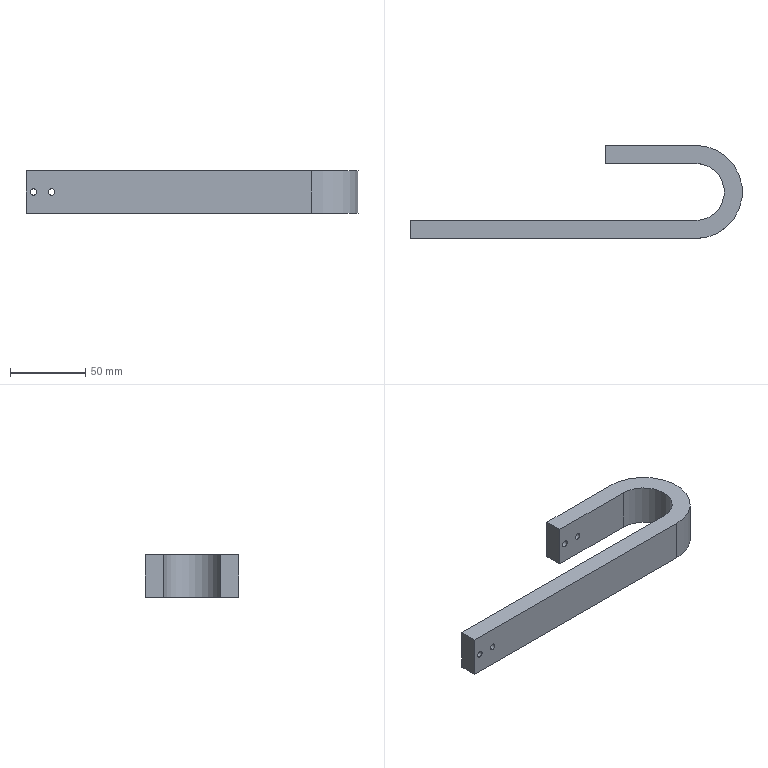Part | NX | features BREP 1 | 1 solid | 18 faces | box 221 x 62 x 28 mm | volume 109724 mm3 | cylinder 10 | plane 8 | commonest cylinder face diameters 4.2 x8 38 x1 62 x1
STEP:
#1=CARTESIAN_POINT('',(280.442,-89.817,14.));
#2=VERTEX_POINT('',#1);
#3=CARTESIAN_POINT('',(276.242,-89.817,14.));
#4=VERTEX_POINT('',#3);
#5=CARTESIAN_POINT('',(278.342,-89.817,14.));
#6=DIRECTION('',(0.,1.,0.));
#7=DIRECTION('',(-1.,0.,0.));
#8=AXIS2_PLACEMENT_3D('',#5,#6,#7);
#9=CIRCLE('',#8,2.1);
#10=EDGE_CURVE('',#2,#4,#9,.T.);
#11=ORIENTED_EDGE('',*,*,#10,.F.);
#12=CARTESIAN_POINT('',(280.442,-77.817,14.));
#13=VERTEX_POINT('',#12);
#14=CARTESIAN_POINT('',(280.442,-92.817,14.));
#15=DIRECTION('',(0.,1.,0.));
#16=VECTOR('',#15,1000.);
#17=LINE('',#14,#16);
#18=EDGE_CURVE('',#2,#13,#17,.T.);
#19=ORIENTED_EDGE('',*,*,#18,.T.);
#20=CARTESIAN_POINT('',(276.242,-77.817,14.));
#21=VERTEX_POINT('',#20);
#22=CARTESIAN_POINT('',(278.342,-77.817,14.));
#23=DIRECTION('',(0.,1.,0.));
#24=DIRECTION('',(-1.,0.,0.));
#25=AXIS2_PLACEMENT_3D('',#22,#23,#24);
#26=CIRCLE('',#25,2.1);
#27=EDGE_CURVE('',#13,#21,#26,.T.);
#28=ORIENTED_EDGE('',*,*,#27,.T.);
#29=CARTESIAN_POINT('',(276.242,-92.817,14.));
#30=DIRECTION('',(0.,1.,0.));
#31=VECTOR('',#30,1000.);
#32=LINE('',#29,#31);
#33=EDGE_CURVE('',#4,#21,#32,.T.);
#34=ORIENTED_EDGE('',*,*,#33,.F.);
#35=EDGE_LOOP('',(#11,#19,#28,#34));
#36=FACE_BOUND('',#35,.T.);
#37=CARTESIAN_POINT('',(278.342,-92.817,14.));
#38=DIRECTION('',(0.,1.,0.));
#39=DIRECTION('',(-1.,0.,0.));
#40=AXIS2_PLACEMENT_3D('',#37,#38,#39);
#41=CYLINDRICAL_SURFACE('',#40,2.1);
#42=ADVANCED_FACE('',(#36),#41,.F.);
#43=CARTESIAN_POINT('',(268.442,-89.817,14.));
#44=VERTEX_POINT('',#43);
#45=CARTESIAN_POINT('',(264.242,-89.817,14.));
#46=VERTEX_POINT('',#45);
#47=CARTESIAN_POINT('',(266.342,-89.817,14.));
#48=DIRECTION('',(0.,1.,0.));
#49=DIRECTION('',(-1.,0.,0.));
#50=AXIS2_PLACEMENT_3D('',#47,#48,#49);
#51=CIRCLE('',#50,2.1);
#52=EDGE_CURVE('',#44,#46,#51,.T.);
#53=ORIENTED_EDGE('',*,*,#52,.F.);
#54=CARTESIAN_POINT('',(268.442,-77.817,14.));
#55=VERTEX_POINT('',#54);
#56=CARTESIAN_POINT('',(268.442,-92.817,14.));
#57=DIRECTION('',(0.,1.,0.));
#58=VECTOR('',#57,1000.);
#59=LINE('',#56,#58);
#60=EDGE_CURVE('',#44,#55,#59,.T.);
#61=ORIENTED_EDGE('',*,*,#60,.T.);
#62=CARTESIAN_POINT('',(264.242,-77.817,14.));
#63=VERTEX_POINT('',#62);
#64=CARTESIAN_POINT('',(266.342,-77.817,14.));
#65=DIRECTION('',(0.,1.,0.));
#66=DIRECTION('',(-1.,0.,0.));
#67=AXIS2_PLACEMENT_3D('',#64,#65,#66);
#68=CIRCLE('',#67,2.1);
#69=EDGE_CURVE('',#55,#63,#68,.T.);
#70=ORIENTED_EDGE('',*,*,#69,.T.);
#71=CARTESIAN_POINT('',(264.242,-92.817,14.));
#72=DIRECTION('',(0.,1.,0.));
#73=VECTOR('',#72,1000.);
#74=LINE('',#71,#73);
#75=EDGE_CURVE('',#46,#63,#74,.T.);
#76=ORIENTED_EDGE('',*,*,#75,.F.);
#77=EDGE_LOOP('',(#53,#61,#70,#76));
#78=FACE_BOUND('',#77,.T.);
#79=CARTESIAN_POINT('',(266.342,-92.817,14.));
#80=DIRECTION('',(0.,1.,0.));
#81=DIRECTION('',(-1.,0.,0.));
#82=AXIS2_PLACEMENT_3D('',#79,#80,#81);
#83=CYLINDRICAL_SURFACE('',#82,2.1);
#84=ADVANCED_FACE('',(#78),#83,.F.);
#85=CARTESIAN_POINT('',(136.342,-139.817,11.9));
#86=VERTEX_POINT('',#85);
#87=CARTESIAN_POINT('',(136.342,-139.817,16.1));
#88=VERTEX_POINT('',#87);
#89=CARTESIAN_POINT('',(136.342,-139.817,14.));
#90=DIRECTION('',(0.,1.,0.));
#91=DIRECTION('',(0.,0.,1.));
#92=AXIS2_PLACEMENT_3D('',#89,#90,#91);
#93=CIRCLE('',#92,2.1);
#94=EDGE_CURVE('',#86,#88,#93,.T.);
#95=ORIENTED_EDGE('',*,*,#94,.F.);
#96=CARTESIAN_POINT('',(136.342,-127.817,11.9));
#97=VERTEX_POINT('',#96);
#98=CARTESIAN_POINT('',(136.342,-142.817,11.9));
#99=DIRECTION('',(0.,1.,0.));
#100=VECTOR('',#99,1000.);
#101=LINE('',#98,#100);
#102=EDGE_CURVE('',#97,#86,#101,.F.);
#103=ORIENTED_EDGE('',*,*,#102,.F.);
#104=CARTESIAN_POINT('',(136.342,-127.817,16.1));
#105=VERTEX_POINT('',#104);
#106=CARTESIAN_POINT('',(136.342,-127.817,14.));
#107=DIRECTION('',(0.,1.,0.));
#108=DIRECTION('',(0.,0.,1.));
#109=AXIS2_PLACEMENT_3D('',#106,#107,#108);
#110=CIRCLE('',#109,2.1);
#111=EDGE_CURVE('',#97,#105,#110,.T.);
#112=ORIENTED_EDGE('',*,*,#111,.T.);
#113=CARTESIAN_POINT('',(136.342,-142.817,16.1));
#114=DIRECTION('',(0.,1.,0.));
#115=VECTOR('',#114,1000.);
#116=LINE('',#113,#115);
#117=EDGE_CURVE('',#105,#88,#116,.F.);
#118=ORIENTED_EDGE('',*,*,#117,.T.);
#119=EDGE_LOOP('',(#95,#103,#112,#118));
#120=FACE_BOUND('',#119,.T.);
#121=CARTESIAN_POINT('',(136.342,-142.817,14.));
#122=DIRECTION('',(0.,1.,0.));
#123=DIRECTION('',(0.,0.,1.));
#124=AXIS2_PLACEMENT_3D('',#121,#122,#123);
#125=CYLINDRICAL_SURFACE('',#124,2.1);
#126=ADVANCED_FACE('',(#120),#125,.F.);
#127=CARTESIAN_POINT('',(148.342,-139.817,11.9));
#128=VERTEX_POINT('',#127);
#129=CARTESIAN_POINT('',(148.342,-139.817,16.1));
#130=VERTEX_POINT('',#129);
#131=CARTESIAN_POINT('',(148.342,-139.817,14.));
#132=DIRECTION('',(0.,1.,0.));
#133=DIRECTION('',(0.,0.,1.));
#134=AXIS2_PLACEMENT_3D('',#131,#132,#133);
#135=CIRCLE('',#134,2.1);
#136=EDGE_CURVE('',#128,#130,#135,.T.);
#137=ORIENTED_EDGE('',*,*,#136,.F.);
#138=CARTESIAN_POINT('',(148.342,-127.817,11.9));
#139=VERTEX_POINT('',#138);
#140=CARTESIAN_POINT('',(148.342,-142.817,11.9));
#141=DIRECTION('',(0.,1.,0.));
#142=VECTOR('',#141,1000.);
#143=LINE('',#140,#142);
#144=EDGE_CURVE('',#139,#128,#143,.F.);
#145=ORIENTED_EDGE('',*,*,#144,.F.);
#146=CARTESIAN_POINT('',(148.342,-127.817,16.1));
#147=VERTEX_POINT('',#146);
#148=CARTESIAN_POINT('',(148.342,-127.817,14.));
#149=DIRECTION('',(0.,1.,0.));
#150=DIRECTION('',(0.,0.,1.));
#151=AXIS2_PLACEMENT_3D('',#148,#149,#150);
#152=CIRCLE('',#151,2.1);
#153=EDGE_CURVE('',#139,#147,#152,.T.);
#154=ORIENTED_EDGE('',*,*,#153,.T.);
#155=CARTESIAN_POINT('',(148.342,-142.817,16.1));
#156=DIRECTION('',(0.,1.,0.));
#157=VECTOR('',#156,1000.);
#158=LINE('',#155,#157);
#159=EDGE_CURVE('',#147,#130,#158,.F.);
#160=ORIENTED_EDGE('',*,*,#159,.T.);
#161=EDGE_LOOP('',(#137,#145,#154,#160));
#162=FACE_BOUND('',#161,.T.);
#163=CARTESIAN_POINT('',(148.342,-142.817,14.));
#164=DIRECTION('',(0.,1.,0.));
#165=DIRECTION('',(0.,0.,1.));
#166=AXIS2_PLACEMENT_3D('',#163,#164,#165);
#167=CYLINDRICAL_SURFACE('',#166,2.1);
#168=ADVANCED_FACE('',(#162),#167,.F.);
#169=CARTESIAN_POINT('',(131.342,-127.817,0.));
#170=VERTEX_POINT('',#169);
#171=CARTESIAN_POINT('',(131.342,-139.817,0.));
#172=VERTEX_POINT('',#171);
#173=CARTESIAN_POINT('',(131.342,-127.817,0.));
#174=DIRECTION('',(0.,-1.,0.));
#175=VECTOR('',#174,1000.);
#176=LINE('',#173,#175);
#177=EDGE_CURVE('',#170,#172,#176,.T.);
#178=ORIENTED_EDGE('',*,*,#177,.T.);
#179=CARTESIAN_POINT('',(131.342,-139.817,28.));
#180=VERTEX_POINT('',#179);
#181=CARTESIAN_POINT('',(131.342,-139.817,28.));
#182=DIRECTION('',(0.,0.,-1.));
#183=VECTOR('',#182,1000.);
#184=LINE('',#181,#183);
#185=EDGE_CURVE('',#180,#172,#184,.T.);
#186=ORIENTED_EDGE('',*,*,#185,.F.);
#187=CARTESIAN_POINT('',(131.342,-127.817,28.));
#188=VERTEX_POINT('',#187);
#189=CARTESIAN_POINT('',(131.342,-127.817,28.));
#190=DIRECTION('',(0.,-1.,0.));
#191=VECTOR('',#190,1000.);
#192=LINE('',#189,#191);
#193=EDGE_CURVE('',#188,#180,#192,.T.);
#194=ORIENTED_EDGE('',*,*,#193,.F.);
#195=CARTESIAN_POINT('',(131.342,-127.817,28.));
#196=DIRECTION('',(0.,0.,-1.));
#197=VECTOR('',#196,1000.);
#198=LINE('',#195,#197);
#199=EDGE_CURVE('',#188,#170,#198,.T.);
#200=ORIENTED_EDGE('',*,*,#199,.T.);
#201=EDGE_LOOP('',(#178,#186,#194,#200));
#202=FACE_BOUND('',#201,.T.);
#203=CARTESIAN_POINT('',(131.342,-127.817,28.));
#204=DIRECTION('',(1.,0.,0.));
#205=DIRECTION('',(0.,1.,0.));
#206=AXIS2_PLACEMENT_3D('',#203,#204,#205);
#207=PLANE('',#206);
#208=ADVANCED_FACE('',(#202),#207,.F.);
#209=CARTESIAN_POINT('',(321.342,-139.817,0.));
#210=VERTEX_POINT('',#209);
#211=CARTESIAN_POINT('',(131.342,-139.817,0.));
#212=DIRECTION('',(1.,0.,0.));
#213=VECTOR('',#212,1000.);
#214=LINE('',#211,#213);
#215=EDGE_CURVE('',#172,#210,#214,.T.);
#216=ORIENTED_EDGE('',*,*,#215,.T.);
#217=CARTESIAN_POINT('',(321.342,-139.817,28.));
#218=VERTEX_POINT('',#217);
#219=CARTESIAN_POINT('',(321.342,-139.817,28.));
#220=DIRECTION('',(0.,0.,-1.));
#221=VECTOR('',#220,1000.);
#222=LINE('',#219,#221);
#223=EDGE_CURVE('',#218,#210,#222,.T.);
#224=ORIENTED_EDGE('',*,*,#223,.F.);
#225=CARTESIAN_POINT('',(131.342,-139.817,28.));
#226=DIRECTION('',(1.,0.,0.));
#227=VECTOR('',#226,1000.);
#228=LINE('',#225,#227);
#229=EDGE_CURVE('',#180,#218,#228,.T.);
#230=ORIENTED_EDGE('',*,*,#229,.F.);
#231=ORIENTED_EDGE('',*,*,#185,.T.);
#232=EDGE_LOOP('',(#216,#224,#230,#231));
#233=FACE_BOUND('',#232,.T.);
#234=CARTESIAN_POINT('',(136.342,-139.817,14.));
#235=DIRECTION('',(0.,1.,0.));
#236=DIRECTION('',(0.,0.,1.));
#237=AXIS2_PLACEMENT_3D('',#234,#235,#236);
#238=CIRCLE('',#237,2.1);
#239=EDGE_CURVE('',#88,#86,#238,.T.);
#240=ORIENTED_EDGE('',*,*,#239,.T.);
#241=ORIENTED_EDGE('',*,*,#94,.T.);
#242=EDGE_LOOP('',(#240,#241));
#243=FACE_BOUND('',#242,.T.);
#244=CARTESIAN_POINT('',(148.342,-139.817,14.));
#245=DIRECTION('',(0.,1.,0.));
#246=DIRECTION('',(0.,0.,1.));
#247=AXIS2_PLACEMENT_3D('',#244,#245,#246);
#248=CIRCLE('',#247,2.1);
#249=EDGE_CURVE('',#130,#128,#248,.T.);
#250=ORIENTED_EDGE('',*,*,#249,.T.);
#251=ORIENTED_EDGE('',*,*,#136,.T.);
#252=EDGE_LOOP('',(#250,#251));
#253=FACE_BOUND('',#252,.T.);
#254=CARTESIAN_POINT('',(131.342,-139.817,28.));
#255=DIRECTION('',(0.,1.,0.));
#256=DIRECTION('',(1.,0.,0.));
#257=AXIS2_PLACEMENT_3D('',#254,#255,#256);
#258=PLANE('',#257);
#259=ADVANCED_FACE('',(#233,#243,#253),#258,.F.);
#260=CARTESIAN_POINT('',(321.342,-77.817,0.));
#261=VERTEX_POINT('',#260);
#262=CARTESIAN_POINT('',(321.342,-108.817,0.));
#263=DIRECTION('',(0.,0.,1.));
#264=DIRECTION('',(1.,0.,0.));
#265=AXIS2_PLACEMENT_3D('',#262,#263,#264);
#266=CIRCLE('',#265,31.);
#267=EDGE_CURVE('',#210,#261,#266,.T.);
#268=ORIENTED_EDGE('',*,*,#267,.T.);
#269=CARTESIAN_POINT('',(321.342,-77.817,28.));
#270=VERTEX_POINT('',#269);
#271=CARTESIAN_POINT('',(321.342,-77.817,28.));
#272=DIRECTION('',(0.,0.,-1.));
#273=VECTOR('',#272,1000.);
#274=LINE('',#271,#273);
#275=EDGE_CURVE('',#270,#261,#274,.T.);
#276=ORIENTED_EDGE('',*,*,#275,.F.);
#277=CARTESIAN_POINT('',(321.342,-108.817,28.));
#278=DIRECTION('',(0.,0.,1.));
#279=DIRECTION('',(1.,0.,0.));
#280=AXIS2_PLACEMENT_3D('',#277,#278,#279);
#281=CIRCLE('',#280,31.);
#282=EDGE_CURVE('',#218,#270,#281,.T.);
#283=ORIENTED_EDGE('',*,*,#282,.F.);
#284=ORIENTED_EDGE('',*,*,#223,.T.);
#285=EDGE_LOOP('',(#268,#276,#283,#284));
#286=FACE_BOUND('',#285,.T.);
#287=CARTESIAN_POINT('',(321.342,-108.817,28.));
#288=DIRECTION('',(0.,0.,-1.));
#289=DIRECTION('',(-1.,0.,0.));
#290=AXIS2_PLACEMENT_3D('',#287,#288,#289);
#291=CYLINDRICAL_SURFACE('',#290,31.);
#292=ADVANCED_FACE('',(#286),#291,.T.);
#293=CARTESIAN_POINT('',(261.342,-77.817,0.));
#294=VERTEX_POINT('',#293);
#295=CARTESIAN_POINT('',(321.342,-77.817,0.));
#296=DIRECTION('',(-1.,0.,0.));
#297=VECTOR('',#296,1000.);
#298=LINE('',#295,#297);
#299=EDGE_CURVE('',#261,#294,#298,.T.);
#300=ORIENTED_EDGE('',*,*,#299,.T.);
#301=CARTESIAN_POINT('',(261.342,-77.817,28.));
#302=VERTEX_POINT('',#301);
#303=CARTESIAN_POINT('',(261.342,-77.817,28.));
#304=DIRECTION('',(0.,0.,-1.));
#305=VECTOR('',#304,1000.);
#306=LINE('',#303,#305);
#307=EDGE_CURVE('',#302,#294,#306,.T.);
#308=ORIENTED_EDGE('',*,*,#307,.F.);
#309=CARTESIAN_POINT('',(321.342,-77.817,28.));
#310=DIRECTION('',(-1.,0.,0.));
#311=VECTOR('',#310,1000.);
#312=LINE('',#309,#311);
#313=EDGE_CURVE('',#270,#302,#312,.T.);
#314=ORIENTED_EDGE('',*,*,#313,.F.);
#315=ORIENTED_EDGE('',*,*,#275,.T.);
#316=EDGE_LOOP('',(#300,#308,#314,#315));
#317=FACE_BOUND('',#316,.T.);
#318=CARTESIAN_POINT('',(278.342,-77.817,14.));
#319=DIRECTION('',(0.,1.,0.));
#320=DIRECTION('',(-1.,0.,0.));
#321=AXIS2_PLACEMENT_3D('',#318,#319,#320);
#322=CIRCLE('',#321,2.1);
#323=EDGE_CURVE('',#21,#13,#322,.T.);
#324=ORIENTED_EDGE('',*,*,#323,.F.);
#325=ORIENTED_EDGE('',*,*,#27,.F.);
#326=EDGE_LOOP('',(#324,#325));
#327=FACE_BOUND('',#326,.T.);
#328=CARTESIAN_POINT('',(266.342,-77.817,14.));
#329=DIRECTION('',(0.,1.,0.));
#330=DIRECTION('',(-1.,0.,0.));
#331=AXIS2_PLACEMENT_3D('',#328,#329,#330);
#332=CIRCLE('',#331,2.1);
#333=EDGE_CURVE('',#63,#55,#332,.T.);
#334=ORIENTED_EDGE('',*,*,#333,.F.);
#335=ORIENTED_EDGE('',*,*,#69,.F.);
#336=EDGE_LOOP('',(#334,#335));
#337=FACE_BOUND('',#336,.T.);
#338=CARTESIAN_POINT('',(321.342,-77.817,28.));
#339=DIRECTION('',(0.,-1.,0.));
#340=DIRECTION('',(-1.,0.,0.));
#341=AXIS2_PLACEMENT_3D('',#338,#339,#340);
#342=PLANE('',#341);
#343=ADVANCED_FACE('',(#317,#327,#337),#342,.F.);
#344=CARTESIAN_POINT('',(261.342,-89.817,0.));
#345=VERTEX_POINT('',#344);
#346=CARTESIAN_POINT('',(261.342,-77.817,0.));
#347=DIRECTION('',(0.,-1.,0.));
#348=VECTOR('',#347,1000.);
#349=LINE('',#346,#348);
#350=EDGE_CURVE('',#294,#345,#349,.T.);
#351=ORIENTED_EDGE('',*,*,#350,.T.);
#352=CARTESIAN_POINT('',(261.342,-89.817,28.));
#353=VERTEX_POINT('',#352);
#354=CARTESIAN_POINT('',(261.342,-89.817,28.));
#355=DIRECTION('',(0.,0.,-1.));
#356=VECTOR('',#355,1000.);
#357=LINE('',#354,#356);
#358=EDGE_CURVE('',#353,#345,#357,.T.);
#359=ORIENTED_EDGE('',*,*,#358,.F.);
#360=CARTESIAN_POINT('',(261.342,-77.817,28.));
#361=DIRECTION('',(0.,-1.,0.));
#362=VECTOR('',#361,1000.);
#363=LINE('',#360,#362);
#364=EDGE_CURVE('',#302,#353,#363,.T.);
#365=ORIENTED_EDGE('',*,*,#364,.F.);
#366=ORIENTED_EDGE('',*,*,#307,.T.);
#367=EDGE_LOOP('',(#351,#359,#365,#366));
#368=FACE_BOUND('',#367,.T.);
#369=CARTESIAN_POINT('',(261.342,-77.817,28.));
#370=DIRECTION('',(1.,0.,0.));
#371=DIRECTION('',(0.,1.,0.));
#372=AXIS2_PLACEMENT_3D('',#369,#370,#371);
#373=PLANE('',#372);
#374=ADVANCED_FACE('',(#368),#373,.F.);
#375=CARTESIAN_POINT('',(321.342,-89.817,0.));
#376=VERTEX_POINT('',#375);
#377=CARTESIAN_POINT('',(321.342,-89.817,0.));
#378=DIRECTION('',(1.,0.,0.));
#379=VECTOR('',#378,1000.);
#380=LINE('',#377,#379);
#381=EDGE_CURVE('',#345,#376,#380,.T.);
#382=ORIENTED_EDGE('',*,*,#381,.T.);
#383=CARTESIAN_POINT('',(321.342,-89.817,28.));
#384=VERTEX_POINT('',#383);
#385=CARTESIAN_POINT('',(321.342,-89.817,28.));
#386=DIRECTION('',(0.,0.,-1.));
#387=VECTOR('',#386,1000.);
#388=LINE('',#385,#387);
#389=EDGE_CURVE('',#384,#376,#388,.T.);
#390=ORIENTED_EDGE('',*,*,#389,.F.);
#391=CARTESIAN_POINT('',(321.342,-89.817,28.));
#392=DIRECTION('',(1.,0.,0.));
#393=VECTOR('',#392,1000.);
#394=LINE('',#391,#393);
#395=EDGE_CURVE('',#353,#384,#394,.T.);
#396=ORIENTED_EDGE('',*,*,#395,.F.);
#397=ORIENTED_EDGE('',*,*,#358,.T.);
#398=EDGE_LOOP('',(#382,#390,#396,#397));
#399=FACE_BOUND('',#398,.T.);
#400=CARTESIAN_POINT('',(278.342,-89.817,14.));
#401=DIRECTION('',(0.,1.,0.));
#402=DIRECTION('',(-1.,0.,0.));
#403=AXIS2_PLACEMENT_3D('',#400,#401,#402);
#404=CIRCLE('',#403,2.1);
#405=EDGE_CURVE('',#4,#2,#404,.T.);
#406=ORIENTED_EDGE('',*,*,#405,.T.);
#407=ORIENTED_EDGE('',*,*,#10,.T.);
#408=EDGE_LOOP('',(#406,#407));
#409=FACE_BOUND('',#408,.T.);
#410=CARTESIAN_POINT('',(266.342,-89.817,14.));
#411=DIRECTION('',(0.,1.,0.));
#412=DIRECTION('',(-1.,0.,0.));
#413=AXIS2_PLACEMENT_3D('',#410,#411,#412);
#414=CIRCLE('',#413,2.1);
#415=EDGE_CURVE('',#46,#44,#414,.T.);
#416=ORIENTED_EDGE('',*,*,#415,.T.);
#417=ORIENTED_EDGE('',*,*,#52,.T.);
#418=EDGE_LOOP('',(#416,#417));
#419=FACE_BOUND('',#418,.T.);
#420=CARTESIAN_POINT('',(321.342,-89.817,28.));
#421=DIRECTION('',(0.,1.,0.));
#422=DIRECTION('',(1.,0.,0.));
#423=AXIS2_PLACEMENT_3D('',#420,#421,#422);
#424=PLANE('',#423);
#425=ADVANCED_FACE('',(#399,#409,#419),#424,.F.);
#426=CARTESIAN_POINT('',(321.342,-127.817,0.));
#427=VERTEX_POINT('',#426);
#428=CARTESIAN_POINT('',(321.342,-108.817,0.));
#429=DIRECTION('',(0.,0.,-1.));
#430=DIRECTION('',(1.,0.,0.));
#431=AXIS2_PLACEMENT_3D('',#428,#429,#430);
#432=CIRCLE('',#431,19.);
#433=EDGE_CURVE('',#376,#427,#432,.T.);
#434=ORIENTED_EDGE('',*,*,#433,.T.);
#435=CARTESIAN_POINT('',(321.342,-127.817,28.));
#436=VERTEX_POINT('',#435);
#437=CARTESIAN_POINT('',(321.342,-127.817,28.));
#438=DIRECTION('',(0.,0.,-1.));
#439=VECTOR('',#438,1000.);
#440=LINE('',#437,#439);
#441=EDGE_CURVE('',#436,#427,#440,.T.);
#442=ORIENTED_EDGE('',*,*,#441,.F.);
#443=CARTESIAN_POINT('',(321.342,-108.817,28.));
#444=DIRECTION('',(0.,0.,-1.));
#445=DIRECTION('',(1.,0.,0.));
#446=AXIS2_PLACEMENT_3D('',#443,#444,#445);
#447=CIRCLE('',#446,19.);
#448=EDGE_CURVE('',#384,#436,#447,.T.);
#449=ORIENTED_EDGE('',*,*,#448,.F.);
#450=ORIENTED_EDGE('',*,*,#389,.T.);
#451=EDGE_LOOP('',(#434,#442,#449,#450));
#452=FACE_BOUND('',#451,.T.);
#453=CARTESIAN_POINT('',(321.342,-108.817,28.));
#454=DIRECTION('',(0.,0.,-1.));
#455=DIRECTION('',(-1.,0.,0.));
#456=AXIS2_PLACEMENT_3D('',#453,#454,#455);
#457=CYLINDRICAL_SURFACE('',#456,19.);
#458=ADVANCED_FACE('',(#452),#457,.F.);
#459=CARTESIAN_POINT('',(131.342,-127.817,0.));
#460=DIRECTION('',(-1.,0.,0.));
#461=VECTOR('',#460,1000.);
#462=LINE('',#459,#461);
#463=EDGE_CURVE('',#427,#170,#462,.T.);
#464=ORIENTED_EDGE('',*,*,#463,.T.);
#465=ORIENTED_EDGE('',*,*,#199,.F.);
#466=CARTESIAN_POINT('',(131.342,-127.817,28.));
#467=DIRECTION('',(-1.,0.,0.));
#468=VECTOR('',#467,1000.);
#469=LINE('',#466,#468);
#470=EDGE_CURVE('',#436,#188,#469,.T.);
#471=ORIENTED_EDGE('',*,*,#470,.F.);
#472=ORIENTED_EDGE('',*,*,#441,.T.);
#473=EDGE_LOOP('',(#464,#465,#471,#472));
#474=FACE_BOUND('',#473,.T.);
#475=CARTESIAN_POINT('',(136.342,-127.817,14.));
#476=DIRECTION('',(0.,1.,0.));
#477=DIRECTION('',(0.,0.,1.));
#478=AXIS2_PLACEMENT_3D('',#475,#476,#477);
#479=CIRCLE('',#478,2.1);
#480=EDGE_CURVE('',#105,#97,#479,.T.);
#481=ORIENTED_EDGE('',*,*,#480,.F.);
#482=ORIENTED_EDGE('',*,*,#111,.F.);
#483=EDGE_LOOP('',(#481,#482));
#484=FACE_BOUND('',#483,.T.);
#485=CARTESIAN_POINT('',(148.342,-127.817,14.));
#486=DIRECTION('',(0.,1.,0.));
#487=DIRECTION('',(0.,0.,1.));
#488=AXIS2_PLACEMENT_3D('',#485,#486,#487);
#489=CIRCLE('',#488,2.1);
#490=EDGE_CURVE('',#147,#139,#489,.T.);
#491=ORIENTED_EDGE('',*,*,#490,.F.);
#492=ORIENTED_EDGE('',*,*,#153,.F.);
#493=EDGE_LOOP('',(#491,#492));
#494=FACE_BOUND('',#493,.T.);
#495=CARTESIAN_POINT('',(131.342,-127.817,28.));
#496=DIRECTION('',(0.,-1.,0.));
#497=DIRECTION('',(0.,0.,-1.));
#498=AXIS2_PLACEMENT_3D('',#495,#496,#497);
#499=PLANE('',#498);
#500=ADVANCED_FACE('',(#474,#484,#494),#499,.F.);
#501=ORIENTED_EDGE('',*,*,#193,.T.);
#502=ORIENTED_EDGE('',*,*,#229,.T.);
#503=ORIENTED_EDGE('',*,*,#282,.T.);
#504=ORIENTED_EDGE('',*,*,#313,.T.);
#505=ORIENTED_EDGE('',*,*,#364,.T.);
#506=ORIENTED_EDGE('',*,*,#395,.T.);
#507=ORIENTED_EDGE('',*,*,#448,.T.);
#508=ORIENTED_EDGE('',*,*,#470,.T.);
#509=EDGE_LOOP('',(#501,#502,#503,#504,#505,#506,#507,#508));
#510=FACE_BOUND('',#509,.T.);
#511=CARTESIAN_POINT('',(321.342,-108.817,28.));
#512=DIRECTION('',(0.,0.,1.));
#513=DIRECTION('',(1.,0.,0.));
#514=AXIS2_PLACEMENT_3D('',#511,#512,#513);
#515=PLANE('',#514);
#516=ADVANCED_FACE('',(#510),#515,.T.);
#517=ORIENTED_EDGE('',*,*,#177,.F.);
#518=ORIENTED_EDGE('',*,*,#463,.F.);
#519=ORIENTED_EDGE('',*,*,#433,.F.);
#520=ORIENTED_EDGE('',*,*,#381,.F.);
#521=ORIENTED_EDGE('',*,*,#350,.F.);
#522=ORIENTED_EDGE('',*,*,#299,.F.);
#523=ORIENTED_EDGE('',*,*,#267,.F.);
#524=ORIENTED_EDGE('',*,*,#215,.F.);
#525=EDGE_LOOP('',(#517,#518,#519,#520,#521,#522,#523,#524));
#526=FACE_BOUND('',#525,.T.);
#527=CARTESIAN_POINT('',(321.342,-108.817,0.));
#528=DIRECTION('',(0.,0.,1.));
#529=DIRECTION('',(1.,0.,0.));
#530=AXIS2_PLACEMENT_3D('',#527,#528,#529);
#531=PLANE('',#530);
#532=ADVANCED_FACE('',(#526),#531,.F.);
#533=ORIENTED_EDGE('',*,*,#144,.T.);
#534=ORIENTED_EDGE('',*,*,#249,.F.);
#535=ORIENTED_EDGE('',*,*,#159,.F.);
#536=ORIENTED_EDGE('',*,*,#490,.T.);
#537=EDGE_LOOP('',(#533,#534,#535,#536));
#538=FACE_BOUND('',#537,.T.);
#539=CARTESIAN_POINT('',(148.342,-142.817,14.));
#540=DIRECTION('',(0.,1.,0.));
#541=DIRECTION('',(0.,0.,1.));
#542=AXIS2_PLACEMENT_3D('',#539,#540,#541);
#543=CYLINDRICAL_SURFACE('',#542,2.1);
#544=ADVANCED_FACE('',(#538),#543,.F.);
#545=ORIENTED_EDGE('',*,*,#102,.T.);
#546=ORIENTED_EDGE('',*,*,#239,.F.);
#547=ORIENTED_EDGE('',*,*,#117,.F.);
#548=ORIENTED_EDGE('',*,*,#480,.T.);
#549=EDGE_LOOP('',(#545,#546,#547,#548));
#550=FACE_BOUND('',#549,.T.);
#551=CARTESIAN_POINT('',(136.342,-142.817,14.));
#552=DIRECTION('',(0.,1.,0.));
#553=DIRECTION('',(0.,0.,1.));
#554=AXIS2_PLACEMENT_3D('',#551,#552,#553);
#555=CYLINDRICAL_SURFACE('',#554,2.1);
#556=ADVANCED_FACE('',(#550),#555,.F.);
#557=ORIENTED_EDGE('',*,*,#60,.F.);
#558=ORIENTED_EDGE('',*,*,#415,.F.);
#559=ORIENTED_EDGE('',*,*,#75,.T.);
#560=ORIENTED_EDGE('',*,*,#333,.T.);
#561=EDGE_LOOP('',(#557,#558,#559,#560));
#562=FACE_BOUND('',#561,.T.);
#563=CARTESIAN_POINT('',(266.342,-92.817,14.));
#564=DIRECTION('',(0.,1.,0.));
#565=DIRECTION('',(-1.,0.,0.));
#566=AXIS2_PLACEMENT_3D('',#563,#564,#565);
#567=CYLINDRICAL_SURFACE('',#566,2.1);
#568=ADVANCED_FACE('',(#562),#567,.F.);
#569=ORIENTED_EDGE('',*,*,#18,.F.);
#570=ORIENTED_EDGE('',*,*,#405,.F.);
#571=ORIENTED_EDGE('',*,*,#33,.T.);
#572=ORIENTED_EDGE('',*,*,#323,.T.);
#573=EDGE_LOOP('',(#569,#570,#571,#572));
#574=FACE_BOUND('',#573,.T.);
#575=CARTESIAN_POINT('',(278.342,-92.817,14.));
#576=DIRECTION('',(0.,1.,0.));
#577=DIRECTION('',(-1.,0.,0.));
#578=AXIS2_PLACEMENT_3D('',#575,#576,#577);
#579=CYLINDRICAL_SURFACE('',#578,2.1);
#580=ADVANCED_FACE('',(#574),#579,.F.);
#581=CLOSED_SHELL('',(#42,#84,#126,#168,#208,#259,#292,#343,#374,#425,#458,#500,#516,#532,#544,#556,#568,#580));
#582=MANIFOLD_SOLID_BREP('',#581);
#583=(LENGTH_UNIT()NAMED_UNIT(*)SI_UNIT(.MILLI.,.METRE.));
#584=UNCERTAINTY_MEASURE_WITH_UNIT(LENGTH_MEASURE(0.00001),#583,'','');
#585=(NAMED_UNIT(*)PLANE_ANGLE_UNIT()SI_UNIT($,.RADIAN.));
#586=(NAMED_UNIT(*)SI_UNIT($,.STERADIAN.)SOLID_ANGLE_UNIT());
#587=(GEOMETRIC_REPRESENTATION_CONTEXT(3)GLOBAL_UNCERTAINTY_ASSIGNED_CONTEXT((#584))GLOBAL_UNIT_ASSIGNED_CONTEXT((#583,#585,#586))REPRESENTATION_CONTEXT('',''));
#588=ADVANCED_BREP_SHAPE_REPRESENTATION('',(#582),#587);